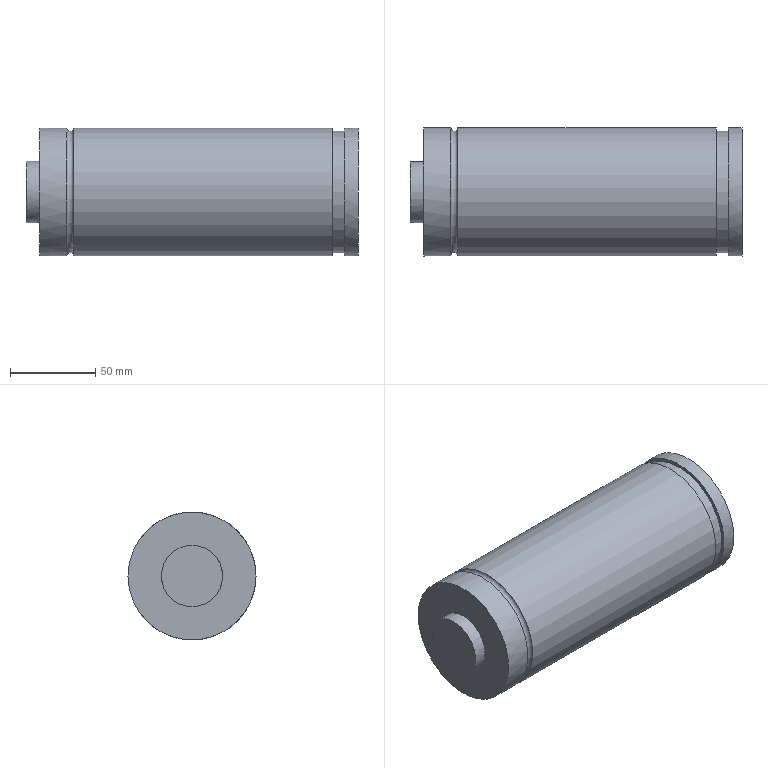Part | NX | features MAIN_BODY 2 | 1 solid | 11 faces | box 195 x 75.2 x 75.2 mm | volume 834025 mm3 | cylinder 5 | plane 5 | torus 1 | commonest cylinder face diameters 75.2 x3 36 x1 71.2 x1
STEP:
#1=CARTESIAN_POINT('',(-409.,217.6,-295.));
#2=VERTEX_POINT('',#1);
#3=CARTESIAN_POINT('',(-409.,180.,-295.));
#4=DIRECTION('',(1.,0.,0.));
#5=DIRECTION('',(0.,1.,0.));
#6=AXIS2_PLACEMENT_3D('',#3,#4,#5);
#7=CIRCLE('',#6,37.6);
#8=EDGE_CURVE('',#2,#2,#7,.F.);
#9=ORIENTED_EDGE('',*,*,#8,.T.);
#10=EDGE_LOOP('',(#9));
#11=FACE_BOUND('',#10,.T.);
#12=CARTESIAN_POINT('',(-561.,217.6,-295.));
#13=VERTEX_POINT('',#12);
#14=CARTESIAN_POINT('',(-561.,180.,-295.));
#15=DIRECTION('',(1.,0.,0.));
#16=DIRECTION('',(0.,1.,0.));
#17=AXIS2_PLACEMENT_3D('',#14,#15,#16);
#18=CIRCLE('',#17,37.6);
#19=EDGE_CURVE('',#13,#13,#18,.T.);
#20=ORIENTED_EDGE('',*,*,#19,.T.);
#21=EDGE_LOOP('',(#20));
#22=FACE_BOUND('',#21,.T.);
#23=CARTESIAN_POINT('',(-581.,180.,-295.));
#24=DIRECTION('',(1.,0.,0.));
#25=DIRECTION('',(0.,1.,0.));
#26=AXIS2_PLACEMENT_3D('',#23,#24,#25);
#27=CYLINDRICAL_SURFACE('',#26,37.6);
#28=ADVANCED_FACE('',(#11,#22),#27,.T.);
#29=CARTESIAN_POINT('',(-581.,142.4,-295.));
#30=VERTEX_POINT('',#29);
#31=CARTESIAN_POINT('',(-581.,180.,-295.));
#32=DIRECTION('',(-1.,0.,0.));
#33=DIRECTION('',(0.,-1.,0.));
#34=AXIS2_PLACEMENT_3D('',#31,#32,#33);
#35=CIRCLE('',#34,37.6);
#36=EDGE_CURVE('',#30,#30,#35,.T.);
#37=ORIENTED_EDGE('',*,*,#36,.T.);
#38=EDGE_LOOP('',(#37));
#39=FACE_BOUND('',#38,.T.);
#40=CARTESIAN_POINT('',(-581.,162.,-295.));
#41=VERTEX_POINT('',#40);
#42=CARTESIAN_POINT('',(-581.,180.,-295.));
#43=DIRECTION('',(-1.,0.,0.));
#44=DIRECTION('',(0.,-1.,0.));
#45=AXIS2_PLACEMENT_3D('',#42,#43,#44);
#46=CIRCLE('',#45,18.);
#47=EDGE_CURVE('',#41,#41,#46,.T.);
#48=ORIENTED_EDGE('',*,*,#47,.F.);
#49=EDGE_LOOP('',(#48));
#50=FACE_BOUND('',#49,.T.);
#51=CARTESIAN_POINT('',(-581.,180.,-295.));
#52=DIRECTION('',(-1.,0.,0.));
#53=DIRECTION('',(0.,-1.,0.));
#54=AXIS2_PLACEMENT_3D('',#51,#52,#53);
#55=PLANE('',#54);
#56=ADVANCED_FACE('',(#39,#50),#55,.T.);
#57=CARTESIAN_POINT('',(-565.,217.6,-295.));
#58=VERTEX_POINT('',#57);
#59=CARTESIAN_POINT('',(-565.,180.,-295.));
#60=DIRECTION('',(1.,0.,0.));
#61=DIRECTION('',(0.,1.,0.));
#62=AXIS2_PLACEMENT_3D('',#59,#60,#61);
#63=CIRCLE('',#62,37.6);
#64=EDGE_CURVE('',#58,#58,#63,.F.);
#65=ORIENTED_EDGE('',*,*,#64,.T.);
#66=EDGE_LOOP('',(#65));
#67=FACE_BOUND('',#66,.T.);
#68=ORIENTED_EDGE('',*,*,#36,.F.);
#69=EDGE_LOOP('',(#68));
#70=FACE_BOUND('',#69,.T.);
#71=CARTESIAN_POINT('',(-581.,180.,-295.));
#72=DIRECTION('',(1.,0.,0.));
#73=DIRECTION('',(0.,1.,0.));
#74=AXIS2_PLACEMENT_3D('',#71,#72,#73);
#75=CYLINDRICAL_SURFACE('',#74,37.6);
#76=ADVANCED_FACE('',(#67,#70),#75,.T.);
#77=ORIENTED_EDGE('',*,*,#47,.T.);
#78=EDGE_LOOP('',(#77));
#79=FACE_BOUND('',#78,.T.);
#80=CARTESIAN_POINT('',(-589.,180.,-277.));
#81=VERTEX_POINT('',#80);
#82=CARTESIAN_POINT('',(-589.,180.,-295.));
#83=DIRECTION('',(-1.,0.,0.));
#84=DIRECTION('',(0.,0.,1.));
#85=AXIS2_PLACEMENT_3D('',#82,#83,#84);
#86=CIRCLE('',#85,18.);
#87=EDGE_CURVE('',#81,#81,#86,.T.);
#88=ORIENTED_EDGE('',*,*,#87,.F.);
#89=EDGE_LOOP('',(#88));
#90=FACE_BOUND('',#89,.T.);
#91=CARTESIAN_POINT('',(-584.,180.,-295.));
#92=DIRECTION('',(1.,0.,0.));
#93=DIRECTION('',(0.,1.,0.));
#94=AXIS2_PLACEMENT_3D('',#91,#92,#93);
#95=CYLINDRICAL_SURFACE('',#94,18.);
#96=ADVANCED_FACE('',(#79,#90),#95,.T.);
#97=ORIENTED_EDGE('',*,*,#64,.F.);
#98=EDGE_LOOP('',(#97));
#99=FACE_BOUND('',#98,.T.);
#100=ORIENTED_EDGE('',*,*,#19,.F.);
#101=EDGE_LOOP('',(#100));
#102=FACE_BOUND('',#101,.T.);
#103=CARTESIAN_POINT('',(-563.,180.,-295.));
#104=DIRECTION('',(1.,0.,0.));
#105=DIRECTION('',(0.,1.,0.));
#106=AXIS2_PLACEMENT_3D('',#103,#104,#105);
#107=TOROIDAL_SURFACE('',#106,37.6,2.);
#108=ADVANCED_FACE('',(#99,#102),#107,.F.);
#109=CARTESIAN_POINT('',(-409.,144.4,-295.));
#110=VERTEX_POINT('',#109);
#111=CARTESIAN_POINT('',(-409.,180.,-295.));
#112=DIRECTION('',(-1.,0.,0.));
#113=DIRECTION('',(0.,-1.,0.));
#114=AXIS2_PLACEMENT_3D('',#111,#112,#113);
#115=CIRCLE('',#114,35.6);
#116=EDGE_CURVE('',#110,#110,#115,.T.);
#117=ORIENTED_EDGE('',*,*,#116,.T.);
#118=EDGE_LOOP('',(#117));
#119=FACE_BOUND('',#118,.T.);
#120=ORIENTED_EDGE('',*,*,#8,.F.);
#121=EDGE_LOOP('',(#120));
#122=FACE_BOUND('',#121,.T.);
#123=CARTESIAN_POINT('',(-409.,180.,-295.));
#124=DIRECTION('',(1.,0.,0.));
#125=DIRECTION('',(0.,1.,0.));
#126=AXIS2_PLACEMENT_3D('',#123,#124,#125);
#127=PLANE('',#126);
#128=ADVANCED_FACE('',(#119,#122),#127,.T.);
#129=CARTESIAN_POINT('',(-402.,144.4,-295.));
#130=VERTEX_POINT('',#129);
#131=CARTESIAN_POINT('',(-402.,180.,-295.));
#132=DIRECTION('',(-1.,0.,0.));
#133=DIRECTION('',(0.,-1.,0.));
#134=AXIS2_PLACEMENT_3D('',#131,#132,#133);
#135=CIRCLE('',#134,35.6);
#136=EDGE_CURVE('',#130,#130,#135,.T.);
#137=ORIENTED_EDGE('',*,*,#136,.F.);
#138=EDGE_LOOP('',(#137));
#139=FACE_BOUND('',#138,.T.);
#140=CARTESIAN_POINT('',(-402.,217.6,-295.));
#141=VERTEX_POINT('',#140);
#142=CARTESIAN_POINT('',(-402.,180.,-295.));
#143=DIRECTION('',(1.,0.,0.));
#144=DIRECTION('',(0.,1.,0.));
#145=AXIS2_PLACEMENT_3D('',#142,#143,#144);
#146=CIRCLE('',#145,37.6);
#147=EDGE_CURVE('',#141,#141,#146,.T.);
#148=ORIENTED_EDGE('',*,*,#147,.F.);
#149=EDGE_LOOP('',(#148));
#150=FACE_BOUND('',#149,.T.);
#151=CARTESIAN_POINT('',(-402.,180.,-295.));
#152=DIRECTION('',(1.,0.,0.));
#153=DIRECTION('',(0.,1.,0.));
#154=AXIS2_PLACEMENT_3D('',#151,#152,#153);
#155=PLANE('',#154);
#156=ADVANCED_FACE('',(#139,#150),#155,.F.);
#157=ORIENTED_EDGE('',*,*,#116,.F.);
#158=EDGE_LOOP('',(#157));
#159=FACE_BOUND('',#158,.T.);
#160=ORIENTED_EDGE('',*,*,#136,.T.);
#161=EDGE_LOOP('',(#160));
#162=FACE_BOUND('',#161,.T.);
#163=CARTESIAN_POINT('',(-402.,180.,-295.));
#164=DIRECTION('',(-1.,0.,0.));
#165=DIRECTION('',(0.,-1.,0.));
#166=AXIS2_PLACEMENT_3D('',#163,#164,#165);
#167=CYLINDRICAL_SURFACE('',#166,35.6);
#168=ADVANCED_FACE('',(#159,#162),#167,.T.);
#169=CARTESIAN_POINT('',(-394.,142.4,-295.));
#170=VERTEX_POINT('',#169);
#171=CARTESIAN_POINT('',(-394.,180.,-295.));
#172=DIRECTION('',(-1.,0.,0.));
#173=DIRECTION('',(0.,-1.,0.));
#174=AXIS2_PLACEMENT_3D('',#171,#172,#173);
#175=CIRCLE('',#174,37.6);
#176=EDGE_CURVE('',#170,#170,#175,.T.);
#177=ORIENTED_EDGE('',*,*,#176,.F.);
#178=EDGE_LOOP('',(#177));
#179=FACE_BOUND('',#178,.T.);
#180=CARTESIAN_POINT('',(-394.,180.,-295.));
#181=DIRECTION('',(-1.,0.,0.));
#182=DIRECTION('',(0.,-1.,0.));
#183=AXIS2_PLACEMENT_3D('',#180,#181,#182);
#184=PLANE('',#183);
#185=ADVANCED_FACE('',(#179),#184,.F.);
#186=ORIENTED_EDGE('',*,*,#147,.T.);
#187=EDGE_LOOP('',(#186));
#188=FACE_BOUND('',#187,.T.);
#189=ORIENTED_EDGE('',*,*,#176,.T.);
#190=EDGE_LOOP('',(#189));
#191=FACE_BOUND('',#190,.T.);
#192=CARTESIAN_POINT('',(-581.,180.,-295.));
#193=DIRECTION('',(1.,0.,0.));
#194=DIRECTION('',(0.,1.,0.));
#195=AXIS2_PLACEMENT_3D('',#192,#193,#194);
#196=CYLINDRICAL_SURFACE('',#195,37.6);
#197=ADVANCED_FACE('',(#188,#191),#196,.T.);
#198=ORIENTED_EDGE('',*,*,#87,.T.);
#199=EDGE_LOOP('',(#198));
#200=FACE_BOUND('',#199,.T.);
#201=CARTESIAN_POINT('',(-589.,180.,-295.));
#202=DIRECTION('',(-1.,0.,0.));
#203=DIRECTION('',(0.,0.,-1.));
#204=AXIS2_PLACEMENT_3D('',#201,#202,#203);
#205=PLANE('',#204);
#206=ADVANCED_FACE('',(#200),#205,.T.);
#207=CLOSED_SHELL('',(#28,#56,#76,#96,#108,#128,#156,#168,#185,#197,#206));
#208=MANIFOLD_SOLID_BREP('',#207);
#209=(LENGTH_UNIT()NAMED_UNIT(*)SI_UNIT(.MILLI.,.METRE.));
#210=UNCERTAINTY_MEASURE_WITH_UNIT(LENGTH_MEASURE(0.00001),#209,'','');
#211=(NAMED_UNIT(*)PLANE_ANGLE_UNIT()SI_UNIT($,.RADIAN.));
#212=(NAMED_UNIT(*)SI_UNIT($,.STERADIAN.)SOLID_ANGLE_UNIT());
#213=(GEOMETRIC_REPRESENTATION_CONTEXT(3)GLOBAL_UNCERTAINTY_ASSIGNED_CONTEXT((#210))GLOBAL_UNIT_ASSIGNED_CONTEXT((#209,#211,#212))REPRESENTATION_CONTEXT('',''));
#214=ADVANCED_BREP_SHAPE_REPRESENTATION('',(#208),#213);